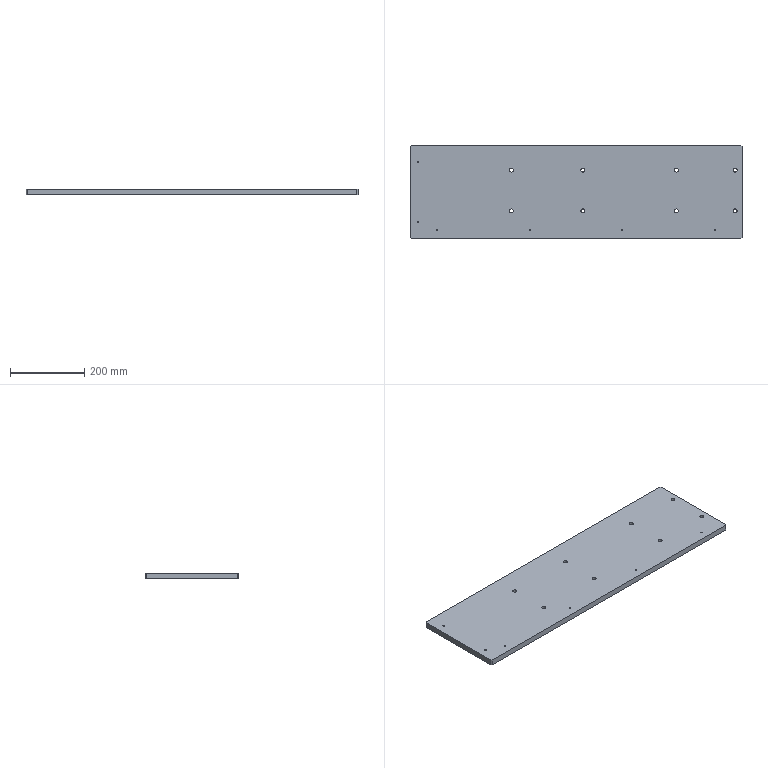Part | NX | features BREP 1 | 1 solid | 38 faces | box 895 x 252 x 16 mm | volume 3596447 mm3 | cylinder 28 | plane 10 | commonest cylinder face diameters 10.5 x16 3.3 x12
STEP:
#1=CARTESIAN_POINT('',(-168.75,59.,16.));
#2=VERTEX_POINT('',#1);
#3=CARTESIAN_POINT('',(-179.25,59.,16.));
#4=VERTEX_POINT('',#3);
#5=CARTESIAN_POINT('',(-174.,59.,16.));
#6=DIRECTION('',(0.,0.,-1.));
#7=DIRECTION('',(-1.,0.,0.));
#8=AXIS2_PLACEMENT_3D('',#5,#6,#7);
#9=CIRCLE('',#8,5.25);
#10=EDGE_CURVE('',#2,#4,#9,.T.);
#11=ORIENTED_EDGE('',*,*,#10,.F.);
#12=CARTESIAN_POINT('',(-168.75,59.,0.));
#13=VERTEX_POINT('',#12);
#14=CARTESIAN_POINT('',(-168.75,59.,0.));
#15=DIRECTION('',(0.,0.,-1.));
#16=VECTOR('',#15,1000.);
#17=LINE('',#14,#16);
#18=EDGE_CURVE('',#2,#13,#17,.T.);
#19=ORIENTED_EDGE('',*,*,#18,.T.);
#20=CARTESIAN_POINT('',(-179.25,59.,0.));
#21=VERTEX_POINT('',#20);
#22=CARTESIAN_POINT('',(-174.,59.,0.));
#23=DIRECTION('',(0.,0.,-1.));
#24=DIRECTION('',(-1.,0.,0.));
#25=AXIS2_PLACEMENT_3D('',#22,#23,#24);
#26=CIRCLE('',#25,5.25);
#27=EDGE_CURVE('',#13,#21,#26,.T.);
#28=ORIENTED_EDGE('',*,*,#27,.T.);
#29=CARTESIAN_POINT('',(-179.25,59.,0.));
#30=DIRECTION('',(0.,0.,-1.));
#31=VECTOR('',#30,1000.);
#32=LINE('',#29,#31);
#33=EDGE_CURVE('',#4,#21,#32,.T.);
#34=ORIENTED_EDGE('',*,*,#33,.F.);
#35=EDGE_LOOP('',(#11,#19,#28,#34));
#36=FACE_BOUND('',#35,.T.);
#37=CARTESIAN_POINT('',(-174.,59.,0.));
#38=DIRECTION('',(0.,0.,-1.));
#39=DIRECTION('',(-1.,0.,0.));
#40=AXIS2_PLACEMENT_3D('',#37,#38,#39);
#41=CYLINDRICAL_SURFACE('',#40,5.25);
#42=ADVANCED_FACE('',(#36),#41,.F.);
#43=CARTESIAN_POINT('',(-168.75,-51.,16.));
#44=VERTEX_POINT('',#43);
#45=CARTESIAN_POINT('',(-179.25,-51.,16.));
#46=VERTEX_POINT('',#45);
#47=CARTESIAN_POINT('',(-174.,-51.,16.));
#48=DIRECTION('',(0.,0.,-1.));
#49=DIRECTION('',(-1.,0.,0.));
#50=AXIS2_PLACEMENT_3D('',#47,#48,#49);
#51=CIRCLE('',#50,5.25);
#52=EDGE_CURVE('',#44,#46,#51,.T.);
#53=ORIENTED_EDGE('',*,*,#52,.F.);
#54=CARTESIAN_POINT('',(-168.75,-51.,0.));
#55=VERTEX_POINT('',#54);
#56=CARTESIAN_POINT('',(-168.75,-51.,0.));
#57=DIRECTION('',(0.,0.,-1.));
#58=VECTOR('',#57,1000.);
#59=LINE('',#56,#58);
#60=EDGE_CURVE('',#44,#55,#59,.T.);
#61=ORIENTED_EDGE('',*,*,#60,.T.);
#62=CARTESIAN_POINT('',(-179.25,-51.,0.));
#63=VERTEX_POINT('',#62);
#64=CARTESIAN_POINT('',(-174.,-51.,0.));
#65=DIRECTION('',(0.,0.,-1.));
#66=DIRECTION('',(-1.,0.,0.));
#67=AXIS2_PLACEMENT_3D('',#64,#65,#66);
#68=CIRCLE('',#67,5.25);
#69=EDGE_CURVE('',#55,#63,#68,.T.);
#70=ORIENTED_EDGE('',*,*,#69,.T.);
#71=CARTESIAN_POINT('',(-179.25,-51.,0.));
#72=DIRECTION('',(0.,0.,-1.));
#73=VECTOR('',#72,1000.);
#74=LINE('',#71,#73);
#75=EDGE_CURVE('',#46,#63,#74,.T.);
#76=ORIENTED_EDGE('',*,*,#75,.F.);
#77=EDGE_LOOP('',(#53,#61,#70,#76));
#78=FACE_BOUND('',#77,.T.);
#79=CARTESIAN_POINT('',(-174.,-51.,0.));
#80=DIRECTION('',(0.,0.,-1.));
#81=DIRECTION('',(-1.,0.,0.));
#82=AXIS2_PLACEMENT_3D('',#79,#80,#81);
#83=CYLINDRICAL_SURFACE('',#82,5.25);
#84=ADVANCED_FACE('',(#78),#83,.F.);
#85=CARTESIAN_POINT('',(23.75,59.,16.));
#86=VERTEX_POINT('',#85);
#87=CARTESIAN_POINT('',(13.25,59.,16.));
#88=VERTEX_POINT('',#87);
#89=CARTESIAN_POINT('',(18.5,59.,16.));
#90=DIRECTION('',(0.,0.,-1.));
#91=DIRECTION('',(-1.,0.,0.));
#92=AXIS2_PLACEMENT_3D('',#89,#90,#91);
#93=CIRCLE('',#92,5.25);
#94=EDGE_CURVE('',#86,#88,#93,.T.);
#95=ORIENTED_EDGE('',*,*,#94,.F.);
#96=CARTESIAN_POINT('',(23.75,59.,0.));
#97=VERTEX_POINT('',#96);
#98=CARTESIAN_POINT('',(23.75,59.,0.));
#99=DIRECTION('',(0.,0.,-1.));
#100=VECTOR('',#99,1000.);
#101=LINE('',#98,#100);
#102=EDGE_CURVE('',#86,#97,#101,.T.);
#103=ORIENTED_EDGE('',*,*,#102,.T.);
#104=CARTESIAN_POINT('',(13.25,59.,0.));
#105=VERTEX_POINT('',#104);
#106=CARTESIAN_POINT('',(18.5,59.,0.));
#107=DIRECTION('',(0.,0.,-1.));
#108=DIRECTION('',(-1.,0.,0.));
#109=AXIS2_PLACEMENT_3D('',#106,#107,#108);
#110=CIRCLE('',#109,5.25);
#111=EDGE_CURVE('',#97,#105,#110,.T.);
#112=ORIENTED_EDGE('',*,*,#111,.T.);
#113=CARTESIAN_POINT('',(13.25,59.,0.));
#114=DIRECTION('',(0.,0.,-1.));
#115=VECTOR('',#114,1000.);
#116=LINE('',#113,#115);
#117=EDGE_CURVE('',#88,#105,#116,.T.);
#118=ORIENTED_EDGE('',*,*,#117,.F.);
#119=EDGE_LOOP('',(#95,#103,#112,#118));
#120=FACE_BOUND('',#119,.T.);
#121=CARTESIAN_POINT('',(18.5,59.,0.));
#122=DIRECTION('',(0.,0.,-1.));
#123=DIRECTION('',(-1.,0.,0.));
#124=AXIS2_PLACEMENT_3D('',#121,#122,#123);
#125=CYLINDRICAL_SURFACE('',#124,5.25);
#126=ADVANCED_FACE('',(#120),#125,.F.);
#127=CARTESIAN_POINT('',(23.75,-51.,16.));
#128=VERTEX_POINT('',#127);
#129=CARTESIAN_POINT('',(13.25,-51.,16.));
#130=VERTEX_POINT('',#129);
#131=CARTESIAN_POINT('',(18.5,-51.,16.));
#132=DIRECTION('',(0.,0.,-1.));
#133=DIRECTION('',(-1.,0.,0.));
#134=AXIS2_PLACEMENT_3D('',#131,#132,#133);
#135=CIRCLE('',#134,5.25);
#136=EDGE_CURVE('',#128,#130,#135,.T.);
#137=ORIENTED_EDGE('',*,*,#136,.F.);
#138=CARTESIAN_POINT('',(23.75,-51.,0.));
#139=VERTEX_POINT('',#138);
#140=CARTESIAN_POINT('',(23.75,-51.,0.));
#141=DIRECTION('',(0.,0.,-1.));
#142=VECTOR('',#141,1000.);
#143=LINE('',#140,#142);
#144=EDGE_CURVE('',#128,#139,#143,.T.);
#145=ORIENTED_EDGE('',*,*,#144,.T.);
#146=CARTESIAN_POINT('',(13.25,-51.,0.));
#147=VERTEX_POINT('',#146);
#148=CARTESIAN_POINT('',(18.5,-51.,0.));
#149=DIRECTION('',(0.,0.,-1.));
#150=DIRECTION('',(-1.,0.,0.));
#151=AXIS2_PLACEMENT_3D('',#148,#149,#150);
#152=CIRCLE('',#151,5.25);
#153=EDGE_CURVE('',#139,#147,#152,.T.);
#154=ORIENTED_EDGE('',*,*,#153,.T.);
#155=CARTESIAN_POINT('',(13.25,-51.,0.));
#156=DIRECTION('',(0.,0.,-1.));
#157=VECTOR('',#156,1000.);
#158=LINE('',#155,#157);
#159=EDGE_CURVE('',#130,#147,#158,.T.);
#160=ORIENTED_EDGE('',*,*,#159,.F.);
#161=EDGE_LOOP('',(#137,#145,#154,#160));
#162=FACE_BOUND('',#161,.T.);
#163=CARTESIAN_POINT('',(18.5,-51.,0.));
#164=DIRECTION('',(0.,0.,-1.));
#165=DIRECTION('',(-1.,0.,0.));
#166=AXIS2_PLACEMENT_3D('',#163,#164,#165);
#167=CYLINDRICAL_SURFACE('',#166,5.25);
#168=ADVANCED_FACE('',(#162),#167,.F.);
#169=CARTESIAN_POINT('',(275.75,59.,16.));
#170=VERTEX_POINT('',#169);
#171=CARTESIAN_POINT('',(265.25,59.,16.));
#172=VERTEX_POINT('',#171);
#173=CARTESIAN_POINT('',(270.5,59.,16.));
#174=DIRECTION('',(0.,0.,-1.));
#175=DIRECTION('',(-1.,0.,0.));
#176=AXIS2_PLACEMENT_3D('',#173,#174,#175);
#177=CIRCLE('',#176,5.25);
#178=EDGE_CURVE('',#170,#172,#177,.T.);
#179=ORIENTED_EDGE('',*,*,#178,.F.);
#180=CARTESIAN_POINT('',(275.75,59.,0.));
#181=VERTEX_POINT('',#180);
#182=CARTESIAN_POINT('',(275.75,59.,0.));
#183=DIRECTION('',(0.,0.,-1.));
#184=VECTOR('',#183,1000.);
#185=LINE('',#182,#184);
#186=EDGE_CURVE('',#170,#181,#185,.T.);
#187=ORIENTED_EDGE('',*,*,#186,.T.);
#188=CARTESIAN_POINT('',(265.25,59.,0.));
#189=VERTEX_POINT('',#188);
#190=CARTESIAN_POINT('',(270.5,59.,0.));
#191=DIRECTION('',(0.,0.,-1.));
#192=DIRECTION('',(-1.,0.,0.));
#193=AXIS2_PLACEMENT_3D('',#190,#191,#192);
#194=CIRCLE('',#193,5.25);
#195=EDGE_CURVE('',#181,#189,#194,.T.);
#196=ORIENTED_EDGE('',*,*,#195,.T.);
#197=CARTESIAN_POINT('',(265.25,59.,0.));
#198=DIRECTION('',(0.,0.,-1.));
#199=VECTOR('',#198,1000.);
#200=LINE('',#197,#199);
#201=EDGE_CURVE('',#172,#189,#200,.T.);
#202=ORIENTED_EDGE('',*,*,#201,.F.);
#203=EDGE_LOOP('',(#179,#187,#196,#202));
#204=FACE_BOUND('',#203,.T.);
#205=CARTESIAN_POINT('',(270.5,59.,0.));
#206=DIRECTION('',(0.,0.,-1.));
#207=DIRECTION('',(-1.,0.,0.));
#208=AXIS2_PLACEMENT_3D('',#205,#206,#207);
#209=CYLINDRICAL_SURFACE('',#208,5.25);
#210=ADVANCED_FACE('',(#204),#209,.F.);
#211=CARTESIAN_POINT('',(275.75,-51.,16.));
#212=VERTEX_POINT('',#211);
#213=CARTESIAN_POINT('',(265.25,-51.,16.));
#214=VERTEX_POINT('',#213);
#215=CARTESIAN_POINT('',(270.5,-51.,16.));
#216=DIRECTION('',(0.,0.,-1.));
#217=DIRECTION('',(-1.,0.,0.));
#218=AXIS2_PLACEMENT_3D('',#215,#216,#217);
#219=CIRCLE('',#218,5.25);
#220=EDGE_CURVE('',#212,#214,#219,.T.);
#221=ORIENTED_EDGE('',*,*,#220,.F.);
#222=CARTESIAN_POINT('',(275.75,-51.,0.));
#223=VERTEX_POINT('',#222);
#224=CARTESIAN_POINT('',(275.75,-51.,0.));
#225=DIRECTION('',(0.,0.,-1.));
#226=VECTOR('',#225,1000.);
#227=LINE('',#224,#226);
#228=EDGE_CURVE('',#212,#223,#227,.T.);
#229=ORIENTED_EDGE('',*,*,#228,.T.);
#230=CARTESIAN_POINT('',(265.25,-51.,0.));
#231=VERTEX_POINT('',#230);
#232=CARTESIAN_POINT('',(270.5,-51.,0.));
#233=DIRECTION('',(0.,0.,-1.));
#234=DIRECTION('',(-1.,0.,0.));
#235=AXIS2_PLACEMENT_3D('',#232,#233,#234);
#236=CIRCLE('',#235,5.25);
#237=EDGE_CURVE('',#223,#231,#236,.T.);
#238=ORIENTED_EDGE('',*,*,#237,.T.);
#239=CARTESIAN_POINT('',(265.25,-51.,0.));
#240=DIRECTION('',(0.,0.,-1.));
#241=VECTOR('',#240,1000.);
#242=LINE('',#239,#241);
#243=EDGE_CURVE('',#214,#231,#242,.T.);
#244=ORIENTED_EDGE('',*,*,#243,.F.);
#245=EDGE_LOOP('',(#221,#229,#238,#244));
#246=FACE_BOUND('',#245,.T.);
#247=CARTESIAN_POINT('',(270.5,-51.,0.));
#248=DIRECTION('',(0.,0.,-1.));
#249=DIRECTION('',(-1.,0.,0.));
#250=AXIS2_PLACEMENT_3D('',#247,#248,#249);
#251=CYLINDRICAL_SURFACE('',#250,5.25);
#252=ADVANCED_FACE('',(#246),#251,.F.);
#253=CARTESIAN_POINT('',(434.25,-51.,16.));
#254=VERTEX_POINT('',#253);
#255=CARTESIAN_POINT('',(423.75,-51.,16.));
#256=VERTEX_POINT('',#255);
#257=CARTESIAN_POINT('',(429.,-51.,16.));
#258=DIRECTION('',(0.,0.,-1.));
#259=DIRECTION('',(-1.,0.,0.));
#260=AXIS2_PLACEMENT_3D('',#257,#258,#259);
#261=CIRCLE('',#260,5.25);
#262=EDGE_CURVE('',#254,#256,#261,.T.);
#263=ORIENTED_EDGE('',*,*,#262,.F.);
#264=CARTESIAN_POINT('',(434.25,-51.,0.));
#265=VERTEX_POINT('',#264);
#266=CARTESIAN_POINT('',(434.25,-51.,0.));
#267=DIRECTION('',(0.,0.,-1.));
#268=VECTOR('',#267,1000.);
#269=LINE('',#266,#268);
#270=EDGE_CURVE('',#254,#265,#269,.T.);
#271=ORIENTED_EDGE('',*,*,#270,.T.);
#272=CARTESIAN_POINT('',(423.75,-51.,0.));
#273=VERTEX_POINT('',#272);
#274=CARTESIAN_POINT('',(429.,-51.,0.));
#275=DIRECTION('',(0.,0.,-1.));
#276=DIRECTION('',(-1.,0.,0.));
#277=AXIS2_PLACEMENT_3D('',#274,#275,#276);
#278=CIRCLE('',#277,5.25);
#279=EDGE_CURVE('',#265,#273,#278,.T.);
#280=ORIENTED_EDGE('',*,*,#279,.T.);
#281=CARTESIAN_POINT('',(423.75,-51.,0.));
#282=DIRECTION('',(0.,0.,-1.));
#283=VECTOR('',#282,1000.);
#284=LINE('',#281,#283);
#285=EDGE_CURVE('',#256,#273,#284,.T.);
#286=ORIENTED_EDGE('',*,*,#285,.F.);
#287=EDGE_LOOP('',(#263,#271,#280,#286));
#288=FACE_BOUND('',#287,.T.);
#289=CARTESIAN_POINT('',(429.,-51.,0.));
#290=DIRECTION('',(0.,0.,-1.));
#291=DIRECTION('',(-1.,0.,0.));
#292=AXIS2_PLACEMENT_3D('',#289,#290,#291);
#293=CYLINDRICAL_SURFACE('',#292,5.25);
#294=ADVANCED_FACE('',(#288),#293,.F.);
#295=CARTESIAN_POINT('',(434.25,59.,16.));
#296=VERTEX_POINT('',#295);
#297=CARTESIAN_POINT('',(423.75,59.,16.));
#298=VERTEX_POINT('',#297);
#299=CARTESIAN_POINT('',(429.,59.,16.));
#300=DIRECTION('',(0.,0.,-1.));
#301=DIRECTION('',(-1.,0.,0.));
#302=AXIS2_PLACEMENT_3D('',#299,#300,#301);
#303=CIRCLE('',#302,5.25);
#304=EDGE_CURVE('',#296,#298,#303,.T.);
#305=ORIENTED_EDGE('',*,*,#304,.F.);
#306=CARTESIAN_POINT('',(434.25,59.,0.));
#307=VERTEX_POINT('',#306);
#308=CARTESIAN_POINT('',(434.25,59.,0.));
#309=DIRECTION('',(0.,0.,-1.));
#310=VECTOR('',#309,1000.);
#311=LINE('',#308,#310);
#312=EDGE_CURVE('',#296,#307,#311,.T.);
#313=ORIENTED_EDGE('',*,*,#312,.T.);
#314=CARTESIAN_POINT('',(423.75,59.,0.));
#315=VERTEX_POINT('',#314);
#316=CARTESIAN_POINT('',(429.,59.,0.));
#317=DIRECTION('',(0.,0.,-1.));
#318=DIRECTION('',(-1.,0.,0.));
#319=AXIS2_PLACEMENT_3D('',#316,#317,#318);
#320=CIRCLE('',#319,5.25);
#321=EDGE_CURVE('',#307,#315,#320,.T.);
#322=ORIENTED_EDGE('',*,*,#321,.T.);
#323=CARTESIAN_POINT('',(423.75,59.,0.));
#324=DIRECTION('',(0.,0.,-1.));
#325=VECTOR('',#324,1000.);
#326=LINE('',#323,#325);
#327=EDGE_CURVE('',#298,#315,#326,.T.);
#328=ORIENTED_EDGE('',*,*,#327,.F.);
#329=EDGE_LOOP('',(#305,#313,#322,#328));
#330=FACE_BOUND('',#329,.T.);
#331=CARTESIAN_POINT('',(429.,59.,0.));
#332=DIRECTION('',(0.,0.,-1.));
#333=DIRECTION('',(-1.,0.,0.));
#334=AXIS2_PLACEMENT_3D('',#331,#332,#333);
#335=CYLINDRICAL_SURFACE('',#334,5.25);
#336=ADVANCED_FACE('',(#330),#335,.F.);
#337=CARTESIAN_POINT('',(-373.35,-103.5,16.));
#338=VERTEX_POINT('',#337);
#339=CARTESIAN_POINT('',(-376.65,-103.5,16.));
#340=VERTEX_POINT('',#339);
#341=CARTESIAN_POINT('',(-375.,-103.5,16.));
#342=DIRECTION('',(0.,0.,-1.));
#343=DIRECTION('',(-1.,0.,0.));
#344=AXIS2_PLACEMENT_3D('',#341,#342,#343);
#345=CIRCLE('',#344,1.65);
#346=EDGE_CURVE('',#338,#340,#345,.T.);
#347=ORIENTED_EDGE('',*,*,#346,.F.);
#348=CARTESIAN_POINT('',(-373.35,-103.5,0.));
#349=VERTEX_POINT('',#348);
#350=CARTESIAN_POINT('',(-373.35,-103.5,0.));
#351=DIRECTION('',(0.,0.,-1.));
#352=VECTOR('',#351,1000.);
#353=LINE('',#350,#352);
#354=EDGE_CURVE('',#338,#349,#353,.T.);
#355=ORIENTED_EDGE('',*,*,#354,.T.);
#356=CARTESIAN_POINT('',(-376.65,-103.5,0.));
#357=VERTEX_POINT('',#356);
#358=CARTESIAN_POINT('',(-375.,-103.5,0.));
#359=DIRECTION('',(0.,0.,-1.));
#360=DIRECTION('',(-1.,0.,0.));
#361=AXIS2_PLACEMENT_3D('',#358,#359,#360);
#362=CIRCLE('',#361,1.65);
#363=EDGE_CURVE('',#349,#357,#362,.T.);
#364=ORIENTED_EDGE('',*,*,#363,.T.);
#365=CARTESIAN_POINT('',(-376.65,-103.5,0.));
#366=DIRECTION('',(0.,0.,-1.));
#367=VECTOR('',#366,1000.);
#368=LINE('',#365,#367);
#369=EDGE_CURVE('',#340,#357,#368,.T.);
#370=ORIENTED_EDGE('',*,*,#369,.F.);
#371=EDGE_LOOP('',(#347,#355,#364,#370));
#372=FACE_BOUND('',#371,.T.);
#373=CARTESIAN_POINT('',(-375.,-103.5,0.));
#374=DIRECTION('',(0.,0.,-1.));
#375=DIRECTION('',(-1.,0.,0.));
#376=AXIS2_PLACEMENT_3D('',#373,#374,#375);
#377=CYLINDRICAL_SURFACE('',#376,1.65);
#378=ADVANCED_FACE('',(#372),#377,.F.);
#379=CARTESIAN_POINT('',(-123.35,-103.5,16.));
#380=VERTEX_POINT('',#379);
#381=CARTESIAN_POINT('',(-126.65,-103.5,16.));
#382=VERTEX_POINT('',#381);
#383=CARTESIAN_POINT('',(-125.,-103.5,16.));
#384=DIRECTION('',(0.,0.,-1.));
#385=DIRECTION('',(-1.,0.,0.));
#386=AXIS2_PLACEMENT_3D('',#383,#384,#385);
#387=CIRCLE('',#386,1.65);
#388=EDGE_CURVE('',#380,#382,#387,.T.);
#389=ORIENTED_EDGE('',*,*,#388,.F.);
#390=CARTESIAN_POINT('',(-123.35,-103.5,0.));
#391=VERTEX_POINT('',#390);
#392=CARTESIAN_POINT('',(-123.35,-103.5,0.));
#393=DIRECTION('',(0.,0.,-1.));
#394=VECTOR('',#393,1000.);
#395=LINE('',#392,#394);
#396=EDGE_CURVE('',#380,#391,#395,.T.);
#397=ORIENTED_EDGE('',*,*,#396,.T.);
#398=CARTESIAN_POINT('',(-126.65,-103.5,0.));
#399=VERTEX_POINT('',#398);
#400=CARTESIAN_POINT('',(-125.,-103.5,0.));
#401=DIRECTION('',(0.,0.,-1.));
#402=DIRECTION('',(-1.,0.,0.));
#403=AXIS2_PLACEMENT_3D('',#400,#401,#402);
#404=CIRCLE('',#403,1.65);
#405=EDGE_CURVE('',#391,#399,#404,.T.);
#406=ORIENTED_EDGE('',*,*,#405,.T.);
#407=CARTESIAN_POINT('',(-126.65,-103.5,0.));
#408=DIRECTION('',(0.,0.,-1.));
#409=VECTOR('',#408,1000.);
#410=LINE('',#407,#409);
#411=EDGE_CURVE('',#382,#399,#410,.T.);
#412=ORIENTED_EDGE('',*,*,#411,.F.);
#413=EDGE_LOOP('',(#389,#397,#406,#412));
#414=FACE_BOUND('',#413,.T.);
#415=CARTESIAN_POINT('',(-125.,-103.5,0.));
#416=DIRECTION('',(0.,0.,-1.));
#417=DIRECTION('',(-1.,0.,0.));
#418=AXIS2_PLACEMENT_3D('',#415,#416,#417);
#419=CYLINDRICAL_SURFACE('',#418,1.65);
#420=ADVANCED_FACE('',(#414),#419,.F.);
#421=CARTESIAN_POINT('',(126.65,-103.5,16.));
#422=VERTEX_POINT('',#421);
#423=CARTESIAN_POINT('',(123.35,-103.5,16.));
#424=VERTEX_POINT('',#423);
#425=CARTESIAN_POINT('',(125.,-103.5,16.));
#426=DIRECTION('',(0.,0.,-1.));
#427=DIRECTION('',(-1.,0.,0.));
#428=AXIS2_PLACEMENT_3D('',#425,#426,#427);
#429=CIRCLE('',#428,1.65);
#430=EDGE_CURVE('',#422,#424,#429,.T.);
#431=ORIENTED_EDGE('',*,*,#430,.F.);
#432=CARTESIAN_POINT('',(126.65,-103.5,0.));
#433=VERTEX_POINT('',#432);
#434=CARTESIAN_POINT('',(126.65,-103.5,0.));
#435=DIRECTION('',(0.,0.,-1.));
#436=VECTOR('',#435,1000.);
#437=LINE('',#434,#436);
#438=EDGE_CURVE('',#422,#433,#437,.T.);
#439=ORIENTED_EDGE('',*,*,#438,.T.);
#440=CARTESIAN_POINT('',(123.35,-103.5,0.));
#441=VERTEX_POINT('',#440);
#442=CARTESIAN_POINT('',(125.,-103.5,0.));
#443=DIRECTION('',(0.,0.,-1.));
#444=DIRECTION('',(-1.,0.,0.));
#445=AXIS2_PLACEMENT_3D('',#442,#443,#444);
#446=CIRCLE('',#445,1.65);
#447=EDGE_CURVE('',#433,#441,#446,.T.);
#448=ORIENTED_EDGE('',*,*,#447,.T.);
#449=CARTESIAN_POINT('',(123.35,-103.5,0.));
#450=DIRECTION('',(0.,0.,-1.));
#451=VECTOR('',#450,1000.);
#452=LINE('',#449,#451);
#453=EDGE_CURVE('',#424,#441,#452,.T.);
#454=ORIENTED_EDGE('',*,*,#453,.F.);
#455=EDGE_LOOP('',(#431,#439,#448,#454));
#456=FACE_BOUND('',#455,.T.);
#457=CARTESIAN_POINT('',(125.,-103.5,0.));
#458=DIRECTION('',(0.,0.,-1.));
#459=DIRECTION('',(-1.,0.,0.));
#460=AXIS2_PLACEMENT_3D('',#457,#458,#459);
#461=CYLINDRICAL_SURFACE('',#460,1.65);
#462=ADVANCED_FACE('',(#456),#461,.F.);
#463=CARTESIAN_POINT('',(376.65,-103.5,16.));
#464=VERTEX_POINT('',#463);
#465=CARTESIAN_POINT('',(373.35,-103.5,16.));
#466=VERTEX_POINT('',#465);
#467=CARTESIAN_POINT('',(375.,-103.5,16.));
#468=DIRECTION('',(0.,0.,-1.));
#469=DIRECTION('',(-1.,0.,0.));
#470=AXIS2_PLACEMENT_3D('',#467,#468,#469);
#471=CIRCLE('',#470,1.65);
#472=EDGE_CURVE('',#464,#466,#471,.T.);
#473=ORIENTED_EDGE('',*,*,#472,.F.);
#474=CARTESIAN_POINT('',(376.65,-103.5,0.));
#475=VERTEX_POINT('',#474);
#476=CARTESIAN_POINT('',(376.65,-103.5,0.));
#477=DIRECTION('',(0.,0.,-1.));
#478=VECTOR('',#477,1000.);
#479=LINE('',#476,#478);
#480=EDGE_CURVE('',#464,#475,#479,.T.);
#481=ORIENTED_EDGE('',*,*,#480,.T.);
#482=CARTESIAN_POINT('',(373.35,-103.5,0.));
#483=VERTEX_POINT('',#482);
#484=CARTESIAN_POINT('',(375.,-103.5,0.));
#485=DIRECTION('',(0.,0.,-1.));
#486=DIRECTION('',(-1.,0.,0.));
#487=AXIS2_PLACEMENT_3D('',#484,#485,#486);
#488=CIRCLE('',#487,1.65);
#489=EDGE_CURVE('',#475,#483,#488,.T.);
#490=ORIENTED_EDGE('',*,*,#489,.T.);
#491=CARTESIAN_POINT('',(373.35,-103.5,0.));
#492=DIRECTION('',(0.,0.,-1.));
#493=VECTOR('',#492,1000.);
#494=LINE('',#491,#493);
#495=EDGE_CURVE('',#466,#483,#494,.T.);
#496=ORIENTED_EDGE('',*,*,#495,.F.);
#497=EDGE_LOOP('',(#473,#481,#490,#496));
#498=FACE_BOUND('',#497,.T.);
#499=CARTESIAN_POINT('',(375.,-103.5,0.));
#500=DIRECTION('',(0.,0.,-1.));
#501=DIRECTION('',(-1.,0.,0.));
#502=AXIS2_PLACEMENT_3D('',#499,#500,#501);
#503=CYLINDRICAL_SURFACE('',#502,1.65);
#504=ADVANCED_FACE('',(#498),#503,.F.);
#505=CARTESIAN_POINT('',(-423.35,-80.,16.));
#506=VERTEX_POINT('',#505);
#507=CARTESIAN_POINT('',(-426.65,-80.,16.));
#508=VERTEX_POINT('',#507);
#509=CARTESIAN_POINT('',(-425.,-80.,16.));
#510=DIRECTION('',(0.,0.,-1.));
#511=DIRECTION('',(-1.,0.,0.));
#512=AXIS2_PLACEMENT_3D('',#509,#510,#511);
#513=CIRCLE('',#512,1.65);
#514=EDGE_CURVE('',#506,#508,#513,.T.);
#515=ORIENTED_EDGE('',*,*,#514,.F.);
#516=CARTESIAN_POINT('',(-423.35,-80.,0.));
#517=VERTEX_POINT('',#516);
#518=CARTESIAN_POINT('',(-423.35,-80.,0.));
#519=DIRECTION('',(0.,0.,-1.));
#520=VECTOR('',#519,1000.);
#521=LINE('',#518,#520);
#522=EDGE_CURVE('',#506,#517,#521,.T.);
#523=ORIENTED_EDGE('',*,*,#522,.T.);
#524=CARTESIAN_POINT('',(-426.65,-80.,0.));
#525=VERTEX_POINT('',#524);
#526=CARTESIAN_POINT('',(-425.,-80.,0.));
#527=DIRECTION('',(0.,0.,-1.));
#528=DIRECTION('',(-1.,0.,0.));
#529=AXIS2_PLACEMENT_3D('',#526,#527,#528);
#530=CIRCLE('',#529,1.65);
#531=EDGE_CURVE('',#517,#525,#530,.T.);
#532=ORIENTED_EDGE('',*,*,#531,.T.);
#533=CARTESIAN_POINT('',(-426.65,-80.,0.));
#534=DIRECTION('',(0.,0.,-1.));
#535=VECTOR('',#534,1000.);
#536=LINE('',#533,#535);
#537=EDGE_CURVE('',#508,#525,#536,.T.);
#538=ORIENTED_EDGE('',*,*,#537,.F.);
#539=EDGE_LOOP('',(#515,#523,#532,#538));
#540=FACE_BOUND('',#539,.T.);
#541=CARTESIAN_POINT('',(-425.,-80.,0.));
#542=DIRECTION('',(0.,0.,-1.));
#543=DIRECTION('',(-1.,0.,0.));
#544=AXIS2_PLACEMENT_3D('',#541,#542,#543);
#545=CYLINDRICAL_SURFACE('',#544,1.65);
#546=ADVANCED_FACE('',(#540),#545,.F.);
#547=CARTESIAN_POINT('',(-423.35,80.,16.));
#548=VERTEX_POINT('',#547);
#549=CARTESIAN_POINT('',(-426.65,80.,16.));
#550=VERTEX_POINT('',#549);
#551=CARTESIAN_POINT('',(-425.,80.,16.));
#552=DIRECTION('',(0.,0.,-1.));
#553=DIRECTION('',(-1.,0.,0.));
#554=AXIS2_PLACEMENT_3D('',#551,#552,#553);
#555=CIRCLE('',#554,1.65);
#556=EDGE_CURVE('',#548,#550,#555,.T.);
#557=ORIENTED_EDGE('',*,*,#556,.F.);
#558=CARTESIAN_POINT('',(-423.35,80.,0.));
#559=VERTEX_POINT('',#558);
#560=CARTESIAN_POINT('',(-423.35,80.,0.));
#561=DIRECTION('',(0.,0.,-1.));
#562=VECTOR('',#561,1000.);
#563=LINE('',#560,#562);
#564=EDGE_CURVE('',#548,#559,#563,.T.);
#565=ORIENTED_EDGE('',*,*,#564,.T.);
#566=CARTESIAN_POINT('',(-426.65,80.,0.));
#567=VERTEX_POINT('',#566);
#568=CARTESIAN_POINT('',(-425.,80.,0.));
#569=DIRECTION('',(0.,0.,-1.));
#570=DIRECTION('',(-1.,0.,0.));
#571=AXIS2_PLACEMENT_3D('',#568,#569,#570);
#572=CIRCLE('',#571,1.65);
#573=EDGE_CURVE('',#559,#567,#572,.T.);
#574=ORIENTED_EDGE('',*,*,#573,.T.);
#575=CARTESIAN_POINT('',(-426.65,80.,0.));
#576=DIRECTION('',(0.,0.,-1.));
#577=VECTOR('',#576,1000.);
#578=LINE('',#575,#577);
#579=EDGE_CURVE('',#550,#567,#578,.T.);
#580=ORIENTED_EDGE('',*,*,#579,.F.);
#581=EDGE_LOOP('',(#557,#565,#574,#580));
#582=FACE_BOUND('',#581,.T.);
#583=CARTESIAN_POINT('',(-425.,80.,0.));
#584=DIRECTION('',(0.,0.,-1.));
#585=DIRECTION('',(-1.,0.,0.));
#586=AXIS2_PLACEMENT_3D('',#583,#584,#585);
#587=CYLINDRICAL_SURFACE('',#586,1.65);
#588=ADVANCED_FACE('',(#582),#587,.F.);
#589=CARTESIAN_POINT('',(447.5,-123.,16.));
#590=VERTEX_POINT('',#589);
#591=CARTESIAN_POINT('',(447.5,123.,16.));
#592=VERTEX_POINT('',#591);
#593=CARTESIAN_POINT('',(447.5,126.,16.));
#594=DIRECTION('',(0.,1.,0.));
#595=VECTOR('',#594,1000.);
#596=LINE('',#593,#595);
#597=EDGE_CURVE('',#590,#592,#596,.T.);
#598=ORIENTED_EDGE('',*,*,#597,.F.);
#599=CARTESIAN_POINT('',(447.5,-123.,0.));
#600=VERTEX_POINT('',#599);
#601=CARTESIAN_POINT('',(447.5,-123.,16.));
#602=DIRECTION('',(0.,0.,-1.));
#603=VECTOR('',#602,1000.);
#604=LINE('',#601,#603);
#605=EDGE_CURVE('',#590,#600,#604,.T.);
#606=ORIENTED_EDGE('',*,*,#605,.T.);
#607=CARTESIAN_POINT('',(447.5,123.,0.));
#608=VERTEX_POINT('',#607);
#609=CARTESIAN_POINT('',(447.5,126.,0.));
#610=DIRECTION('',(0.,1.,0.));
#611=VECTOR('',#610,1000.);
#612=LINE('',#609,#611);
#613=EDGE_CURVE('',#600,#608,#612,.T.);
#614=ORIENTED_EDGE('',*,*,#613,.T.);
#615=CARTESIAN_POINT('',(447.5,123.,16.));
#616=DIRECTION('',(0.,0.,1.));
#617=VECTOR('',#616,1000.);
#618=LINE('',#615,#617);
#619=EDGE_CURVE('',#608,#592,#618,.T.);
#620=ORIENTED_EDGE('',*,*,#619,.T.);
#621=EDGE_LOOP('',(#598,#606,#614,#620));
#622=FACE_BOUND('',#621,.T.);
#623=CARTESIAN_POINT('',(447.5,126.,16.));
#624=DIRECTION('',(-1.,0.,0.));
#625=DIRECTION('',(0.,0.,1.));
#626=AXIS2_PLACEMENT_3D('',#623,#624,#625);
#627=PLANE('',#626);
#628=ADVANCED_FACE('',(#622),#627,.F.);
#629=CARTESIAN_POINT('',(444.5,126.,0.));
#630=VERTEX_POINT('',#629);
#631=CARTESIAN_POINT('',(-444.5,126.,0.));
#632=VERTEX_POINT('',#631);
#633=CARTESIAN_POINT('',(-447.5,126.,0.));
#634=DIRECTION('',(-1.,0.,0.));
#635=VECTOR('',#634,1000.);
#636=LINE('',#633,#635);
#637=EDGE_CURVE('',#630,#632,#636,.T.);
#638=ORIENTED_EDGE('',*,*,#637,.T.);
#639=CARTESIAN_POINT('',(-444.5,126.,16.));
#640=VERTEX_POINT('',#639);
#641=CARTESIAN_POINT('',(-444.5,126.,16.));
#642=DIRECTION('',(0.,0.,1.));
#643=VECTOR('',#642,1000.);
#644=LINE('',#641,#643);
#645=EDGE_CURVE('',#632,#640,#644,.T.);
#646=ORIENTED_EDGE('',*,*,#645,.T.);
#647=CARTESIAN_POINT('',(444.5,126.,16.));
#648=VERTEX_POINT('',#647);
#649=CARTESIAN_POINT('',(-447.5,126.,16.));
#650=DIRECTION('',(-1.,0.,0.));
#651=VECTOR('',#650,1000.);
#652=LINE('',#649,#651);
#653=EDGE_CURVE('',#648,#640,#652,.T.);
#654=ORIENTED_EDGE('',*,*,#653,.F.);
#655=CARTESIAN_POINT('',(444.5,126.,16.));
#656=DIRECTION('',(0.,0.,-1.));
#657=VECTOR('',#656,1000.);
#658=LINE('',#655,#657);
#659=EDGE_CURVE('',#648,#630,#658,.T.);
#660=ORIENTED_EDGE('',*,*,#659,.T.);
#661=EDGE_LOOP('',(#638,#646,#654,#660));
#662=FACE_BOUND('',#661,.T.);
#663=CARTESIAN_POINT('',(-447.5,126.,16.));
#664=DIRECTION('',(0.,-1.,0.));
#665=DIRECTION('',(0.,0.,-1.));
#666=AXIS2_PLACEMENT_3D('',#663,#664,#665);
#667=PLANE('',#666);
#668=ADVANCED_FACE('',(#662),#667,.F.);
#669=CARTESIAN_POINT('',(-447.5,123.,0.));
#670=VERTEX_POINT('',#669);
#671=CARTESIAN_POINT('',(-447.5,-123.,0.));
#672=VERTEX_POINT('',#671);
#673=CARTESIAN_POINT('',(-447.5,126.,0.));
#674=DIRECTION('',(0.,-1.,0.));
#675=VECTOR('',#674,1000.);
#676=LINE('',#673,#675);
#677=EDGE_CURVE('',#670,#672,#676,.T.);
#678=ORIENTED_EDGE('',*,*,#677,.T.);
#679=CARTESIAN_POINT('',(-447.5,-123.,16.));
#680=VERTEX_POINT('',#679);
#681=CARTESIAN_POINT('',(-447.5,-123.,16.));
#682=DIRECTION('',(0.,0.,1.));
#683=VECTOR('',#682,1000.);
#684=LINE('',#681,#683);
#685=EDGE_CURVE('',#672,#680,#684,.T.);
#686=ORIENTED_EDGE('',*,*,#685,.T.);
#687=CARTESIAN_POINT('',(-447.5,123.,16.));
#688=VERTEX_POINT('',#687);
#689=CARTESIAN_POINT('',(-447.5,126.,16.));
#690=DIRECTION('',(0.,-1.,0.));
#691=VECTOR('',#690,1000.);
#692=LINE('',#689,#691);
#693=EDGE_CURVE('',#688,#680,#692,.T.);
#694=ORIENTED_EDGE('',*,*,#693,.F.);
#695=CARTESIAN_POINT('',(-447.5,123.,16.));
#696=DIRECTION('',(0.,0.,-1.));
#697=VECTOR('',#696,1000.);
#698=LINE('',#695,#697);
#699=EDGE_CURVE('',#688,#670,#698,.T.);
#700=ORIENTED_EDGE('',*,*,#699,.T.);
#701=EDGE_LOOP('',(#678,#686,#694,#700));
#702=FACE_BOUND('',#701,.T.);
#703=CARTESIAN_POINT('',(-447.5,126.,16.));
#704=DIRECTION('',(1.,0.,0.));
#705=DIRECTION('',(0.,1.,0.));
#706=AXIS2_PLACEMENT_3D('',#703,#704,#705);
#707=PLANE('',#706);
#708=ADVANCED_FACE('',(#702),#707,.F.);
#709=CARTESIAN_POINT('',(-444.5,-126.,0.));
#710=VERTEX_POINT('',#709);
#711=CARTESIAN_POINT('',(444.5,-126.,0.));
#712=VERTEX_POINT('',#711);
#713=CARTESIAN_POINT('',(-447.5,-126.,0.));
#714=DIRECTION('',(1.,0.,0.));
#715=VECTOR('',#714,1000.);
#716=LINE('',#713,#715);
#717=EDGE_CURVE('',#710,#712,#716,.T.);
#718=ORIENTED_EDGE('',*,*,#717,.T.);
#719=CARTESIAN_POINT('',(444.5,-126.,16.));
#720=VERTEX_POINT('',#719);
#721=CARTESIAN_POINT('',(444.5,-126.,16.));
#722=DIRECTION('',(0.,0.,1.));
#723=VECTOR('',#722,1000.);
#724=LINE('',#721,#723);
#725=EDGE_CURVE('',#712,#720,#724,.T.);
#726=ORIENTED_EDGE('',*,*,#725,.T.);
#727=CARTESIAN_POINT('',(-444.5,-126.,16.));
#728=VERTEX_POINT('',#727);
#729=CARTESIAN_POINT('',(-447.5,-126.,16.));
#730=DIRECTION('',(1.,0.,0.));
#731=VECTOR('',#730,1000.);
#732=LINE('',#729,#731);
#733=EDGE_CURVE('',#728,#720,#732,.T.);
#734=ORIENTED_EDGE('',*,*,#733,.F.);
#735=CARTESIAN_POINT('',(-444.5,-126.,16.));
#736=DIRECTION('',(0.,0.,-1.));
#737=VECTOR('',#736,1000.);
#738=LINE('',#735,#737);
#739=EDGE_CURVE('',#728,#710,#738,.T.);
#740=ORIENTED_EDGE('',*,*,#739,.T.);
#741=EDGE_LOOP('',(#718,#726,#734,#740));
#742=FACE_BOUND('',#741,.T.);
#743=CARTESIAN_POINT('',(-447.5,-126.,16.));
#744=DIRECTION('',(0.,1.,0.));
#745=DIRECTION('',(1.,0.,0.));
#746=AXIS2_PLACEMENT_3D('',#743,#744,#745);
#747=PLANE('',#746);
#748=ADVANCED_FACE('',(#742),#747,.F.);
#749=ORIENTED_EDGE('',*,*,#733,.T.);
#750=CARTESIAN_POINT('',(446.,-124.5,16.));
#751=DIRECTION('',(0.7071,0.7071,0.));
#752=VECTOR('',#751,1000.);
#753=LINE('',#750,#752);
#754=EDGE_CURVE('',#720,#590,#753,.T.);
#755=ORIENTED_EDGE('',*,*,#754,.T.);
#756=ORIENTED_EDGE('',*,*,#597,.T.);
#757=CARTESIAN_POINT('',(572.,-1.5,16.));
#758=DIRECTION('',(-0.7071,0.7071,0.));
#759=VECTOR('',#758,1000.);
#760=LINE('',#757,#759);
#761=EDGE_CURVE('',#592,#648,#760,.T.);
#762=ORIENTED_EDGE('',*,*,#761,.T.);
#763=ORIENTED_EDGE('',*,*,#653,.T.);
#764=CARTESIAN_POINT('',(-124.5,446.,16.));
#765=DIRECTION('',(-0.7071,-0.7071,0.));
#766=VECTOR('',#765,1000.);
#767=LINE('',#764,#766);
#768=EDGE_CURVE('',#640,#688,#767,.T.);
#769=ORIENTED_EDGE('',*,*,#768,.T.);
#770=ORIENTED_EDGE('',*,*,#693,.T.);
#771=CARTESIAN_POINT('',(1.5,-572.,16.));
#772=DIRECTION('',(0.7071,-0.7071,0.));
#773=VECTOR('',#772,1000.);
#774=LINE('',#771,#773);
#775=EDGE_CURVE('',#680,#728,#774,.T.);
#776=ORIENTED_EDGE('',*,*,#775,.T.);
#777=EDGE_LOOP('',(#749,#755,#756,#762,#763,#769,#770,#776));
#778=FACE_BOUND('',#777,.T.);
#779=CARTESIAN_POINT('',(-174.,59.,16.));
#780=DIRECTION('',(0.,0.,-1.));
#781=DIRECTION('',(-1.,0.,0.));
#782=AXIS2_PLACEMENT_3D('',#779,#780,#781);
#783=CIRCLE('',#782,5.25);
#784=EDGE_CURVE('',#4,#2,#783,.T.);
#785=ORIENTED_EDGE('',*,*,#784,.T.);
#786=ORIENTED_EDGE('',*,*,#10,.T.);
#787=EDGE_LOOP('',(#785,#786));
#788=FACE_BOUND('',#787,.T.);
#789=CARTESIAN_POINT('',(-174.,-51.,16.));
#790=DIRECTION('',(0.,0.,-1.));
#791=DIRECTION('',(-1.,0.,0.));
#792=AXIS2_PLACEMENT_3D('',#789,#790,#791);
#793=CIRCLE('',#792,5.25);
#794=EDGE_CURVE('',#46,#44,#793,.T.);
#795=ORIENTED_EDGE('',*,*,#794,.T.);
#796=ORIENTED_EDGE('',*,*,#52,.T.);
#797=EDGE_LOOP('',(#795,#796));
#798=FACE_BOUND('',#797,.T.);
#799=CARTESIAN_POINT('',(18.5,59.,16.));
#800=DIRECTION('',(0.,0.,-1.));
#801=DIRECTION('',(-1.,0.,0.));
#802=AXIS2_PLACEMENT_3D('',#799,#800,#801);
#803=CIRCLE('',#802,5.25);
#804=EDGE_CURVE('',#88,#86,#803,.T.);
#805=ORIENTED_EDGE('',*,*,#804,.T.);
#806=ORIENTED_EDGE('',*,*,#94,.T.);
#807=EDGE_LOOP('',(#805,#806));
#808=FACE_BOUND('',#807,.T.);
#809=CARTESIAN_POINT('',(18.5,-51.,16.));
#810=DIRECTION('',(0.,0.,-1.));
#811=DIRECTION('',(-1.,0.,0.));
#812=AXIS2_PLACEMENT_3D('',#809,#810,#811);
#813=CIRCLE('',#812,5.25);
#814=EDGE_CURVE('',#130,#128,#813,.T.);
#815=ORIENTED_EDGE('',*,*,#814,.T.);
#816=ORIENTED_EDGE('',*,*,#136,.T.);
#817=EDGE_LOOP('',(#815,#816));
#818=FACE_BOUND('',#817,.T.);
#819=CARTESIAN_POINT('',(270.5,59.,16.));
#820=DIRECTION('',(0.,0.,-1.));
#821=DIRECTION('',(-1.,0.,0.));
#822=AXIS2_PLACEMENT_3D('',#819,#820,#821);
#823=CIRCLE('',#822,5.25);
#824=EDGE_CURVE('',#172,#170,#823,.T.);
#825=ORIENTED_EDGE('',*,*,#824,.T.);
#826=ORIENTED_EDGE('',*,*,#178,.T.);
#827=EDGE_LOOP('',(#825,#826));
#828=FACE_BOUND('',#827,.T.);
#829=CARTESIAN_POINT('',(270.5,-51.,16.));
#830=DIRECTION('',(0.,0.,-1.));
#831=DIRECTION('',(-1.,0.,0.));
#832=AXIS2_PLACEMENT_3D('',#829,#830,#831);
#833=CIRCLE('',#832,5.25);
#834=EDGE_CURVE('',#214,#212,#833,.T.);
#835=ORIENTED_EDGE('',*,*,#834,.T.);
#836=ORIENTED_EDGE('',*,*,#220,.T.);
#837=EDGE_LOOP('',(#835,#836));
#838=FACE_BOUND('',#837,.T.);
#839=CARTESIAN_POINT('',(429.,-51.,16.));
#840=DIRECTION('',(0.,0.,-1.));
#841=DIRECTION('',(-1.,0.,0.));
#842=AXIS2_PLACEMENT_3D('',#839,#840,#841);
#843=CIRCLE('',#842,5.25);
#844=EDGE_CURVE('',#256,#254,#843,.T.);
#845=ORIENTED_EDGE('',*,*,#844,.T.);
#846=ORIENTED_EDGE('',*,*,#262,.T.);
#847=EDGE_LOOP('',(#845,#846));
#848=FACE_BOUND('',#847,.T.);
#849=CARTESIAN_POINT('',(429.,59.,16.));
#850=DIRECTION('',(0.,0.,-1.));
#851=DIRECTION('',(-1.,0.,0.));
#852=AXIS2_PLACEMENT_3D('',#849,#850,#851);
#853=CIRCLE('',#852,5.25);
#854=EDGE_CURVE('',#298,#296,#853,.T.);
#855=ORIENTED_EDGE('',*,*,#854,.T.);
#856=ORIENTED_EDGE('',*,*,#304,.T.);
#857=EDGE_LOOP('',(#855,#856));
#858=FACE_BOUND('',#857,.T.);
#859=CARTESIAN_POINT('',(-375.,-103.5,16.));
#860=DIRECTION('',(0.,0.,-1.));
#861=DIRECTION('',(-1.,0.,0.));
#862=AXIS2_PLACEMENT_3D('',#859,#860,#861);
#863=CIRCLE('',#862,1.65);
#864=EDGE_CURVE('',#340,#338,#863,.T.);
#865=ORIENTED_EDGE('',*,*,#864,.T.);
#866=ORIENTED_EDGE('',*,*,#346,.T.);
#867=EDGE_LOOP('',(#865,#866));
#868=FACE_BOUND('',#867,.T.);
#869=CARTESIAN_POINT('',(-125.,-103.5,16.));
#870=DIRECTION('',(0.,0.,-1.));
#871=DIRECTION('',(-1.,0.,0.));
#872=AXIS2_PLACEMENT_3D('',#869,#870,#871);
#873=CIRCLE('',#872,1.65);
#874=EDGE_CURVE('',#382,#380,#873,.T.);
#875=ORIENTED_EDGE('',*,*,#874,.T.);
#876=ORIENTED_EDGE('',*,*,#388,.T.);
#877=EDGE_LOOP('',(#875,#876));
#878=FACE_BOUND('',#877,.T.);
#879=CARTESIAN_POINT('',(125.,-103.5,16.));
#880=DIRECTION('',(0.,0.,-1.));
#881=DIRECTION('',(-1.,0.,0.));
#882=AXIS2_PLACEMENT_3D('',#879,#880,#881);
#883=CIRCLE('',#882,1.65);
#884=EDGE_CURVE('',#424,#422,#883,.T.);
#885=ORIENTED_EDGE('',*,*,#884,.T.);
#886=ORIENTED_EDGE('',*,*,#430,.T.);
#887=EDGE_LOOP('',(#885,#886));
#888=FACE_BOUND('',#887,.T.);
#889=CARTESIAN_POINT('',(375.,-103.5,16.));
#890=DIRECTION('',(0.,0.,-1.));
#891=DIRECTION('',(-1.,0.,0.));
#892=AXIS2_PLACEMENT_3D('',#889,#890,#891);
#893=CIRCLE('',#892,1.65);
#894=EDGE_CURVE('',#466,#464,#893,.T.);
#895=ORIENTED_EDGE('',*,*,#894,.T.);
#896=ORIENTED_EDGE('',*,*,#472,.T.);
#897=EDGE_LOOP('',(#895,#896));
#898=FACE_BOUND('',#897,.T.);
#899=CARTESIAN_POINT('',(-425.,-80.,16.));
#900=DIRECTION('',(0.,0.,-1.));
#901=DIRECTION('',(-1.,0.,0.));
#902=AXIS2_PLACEMENT_3D('',#899,#900,#901);
#903=CIRCLE('',#902,1.65);
#904=EDGE_CURVE('',#508,#506,#903,.T.);
#905=ORIENTED_EDGE('',*,*,#904,.T.);
#906=ORIENTED_EDGE('',*,*,#514,.T.);
#907=EDGE_LOOP('',(#905,#906));
#908=FACE_BOUND('',#907,.T.);
#909=CARTESIAN_POINT('',(-425.,80.,16.));
#910=DIRECTION('',(0.,0.,-1.));
#911=DIRECTION('',(-1.,0.,0.));
#912=AXIS2_PLACEMENT_3D('',#909,#910,#911);
#913=CIRCLE('',#912,1.65);
#914=EDGE_CURVE('',#550,#548,#913,.T.);
#915=ORIENTED_EDGE('',*,*,#914,.T.);
#916=ORIENTED_EDGE('',*,*,#556,.T.);
#917=EDGE_LOOP('',(#915,#916));
#918=FACE_BOUND('',#917,.T.);
#919=CARTESIAN_POINT('',(447.5,-126.,16.));
#920=DIRECTION('',(0.,0.,1.));
#921=DIRECTION('',(1.,0.,0.));
#922=AXIS2_PLACEMENT_3D('',#919,#920,#921);
#923=PLANE('',#922);
#924=ADVANCED_FACE('',(#778,#788,#798,#808,#818,#828,#838,#848,#858,#868,#878,#888,#898,#908,#918),#923,.T.);
#925=ORIENTED_EDGE('',*,*,#613,.F.);
#926=CARTESIAN_POINT('',(447.5,-123.,0.));
#927=DIRECTION('',(-0.7071,-0.7071,0.));
#928=VECTOR('',#927,1000.);
#929=LINE('',#926,#928);
#930=EDGE_CURVE('',#600,#712,#929,.T.);
#931=ORIENTED_EDGE('',*,*,#930,.T.);
#932=ORIENTED_EDGE('',*,*,#717,.F.);
#933=CARTESIAN_POINT('',(-444.5,-126.,0.));
#934=DIRECTION('',(-0.7071,0.7071,0.));
#935=VECTOR('',#934,1000.);
#936=LINE('',#933,#935);
#937=EDGE_CURVE('',#710,#672,#936,.T.);
#938=ORIENTED_EDGE('',*,*,#937,.T.);
#939=ORIENTED_EDGE('',*,*,#677,.F.);
#940=CARTESIAN_POINT('',(-447.5,123.,0.));
#941=DIRECTION('',(0.7071,0.7071,0.));
#942=VECTOR('',#941,1000.);
#943=LINE('',#940,#942);
#944=EDGE_CURVE('',#670,#632,#943,.T.);
#945=ORIENTED_EDGE('',*,*,#944,.T.);
#946=ORIENTED_EDGE('',*,*,#637,.F.);
#947=CARTESIAN_POINT('',(444.5,126.,0.));
#948=DIRECTION('',(0.7071,-0.7071,0.));
#949=VECTOR('',#948,1000.);
#950=LINE('',#947,#949);
#951=EDGE_CURVE('',#630,#608,#950,.T.);
#952=ORIENTED_EDGE('',*,*,#951,.T.);
#953=EDGE_LOOP('',(#925,#931,#932,#938,#939,#945,#946,#952));
#954=FACE_BOUND('',#953,.T.);
#955=CARTESIAN_POINT('',(-174.,59.,0.));
#956=DIRECTION('',(0.,0.,-1.));
#957=DIRECTION('',(-1.,0.,0.));
#958=AXIS2_PLACEMENT_3D('',#955,#956,#957);
#959=CIRCLE('',#958,5.25);
#960=EDGE_CURVE('',#21,#13,#959,.T.);
#961=ORIENTED_EDGE('',*,*,#960,.F.);
#962=ORIENTED_EDGE('',*,*,#27,.F.);
#963=EDGE_LOOP('',(#961,#962));
#964=FACE_BOUND('',#963,.T.);
#965=CARTESIAN_POINT('',(-174.,-51.,0.));
#966=DIRECTION('',(0.,0.,-1.));
#967=DIRECTION('',(-1.,0.,0.));
#968=AXIS2_PLACEMENT_3D('',#965,#966,#967);
#969=CIRCLE('',#968,5.25);
#970=EDGE_CURVE('',#63,#55,#969,.T.);
#971=ORIENTED_EDGE('',*,*,#970,.F.);
#972=ORIENTED_EDGE('',*,*,#69,.F.);
#973=EDGE_LOOP('',(#971,#972));
#974=FACE_BOUND('',#973,.T.);
#975=CARTESIAN_POINT('',(18.5,59.,0.));
#976=DIRECTION('',(0.,0.,-1.));
#977=DIRECTION('',(-1.,0.,0.));
#978=AXIS2_PLACEMENT_3D('',#975,#976,#977);
#979=CIRCLE('',#978,5.25);
#980=EDGE_CURVE('',#105,#97,#979,.T.);
#981=ORIENTED_EDGE('',*,*,#980,.F.);
#982=ORIENTED_EDGE('',*,*,#111,.F.);
#983=EDGE_LOOP('',(#981,#982));
#984=FACE_BOUND('',#983,.T.);
#985=CARTESIAN_POINT('',(18.5,-51.,0.));
#986=DIRECTION('',(0.,0.,-1.));
#987=DIRECTION('',(-1.,0.,0.));
#988=AXIS2_PLACEMENT_3D('',#985,#986,#987);
#989=CIRCLE('',#988,5.25);
#990=EDGE_CURVE('',#147,#139,#989,.T.);
#991=ORIENTED_EDGE('',*,*,#990,.F.);
#992=ORIENTED_EDGE('',*,*,#153,.F.);
#993=EDGE_LOOP('',(#991,#992));
#994=FACE_BOUND('',#993,.T.);
#995=CARTESIAN_POINT('',(270.5,59.,0.));
#996=DIRECTION('',(0.,0.,-1.));
#997=DIRECTION('',(-1.,0.,0.));
#998=AXIS2_PLACEMENT_3D('',#995,#996,#997);
#999=CIRCLE('',#998,5.25);
#1000=EDGE_CURVE('',#189,#181,#999,.T.);
#1001=ORIENTED_EDGE('',*,*,#1000,.F.);
#1002=ORIENTED_EDGE('',*,*,#195,.F.);
#1003=EDGE_LOOP('',(#1001,#1002));
#1004=FACE_BOUND('',#1003,.T.);
#1005=CARTESIAN_POINT('',(270.5,-51.,0.));
#1006=DIRECTION('',(0.,0.,-1.));
#1007=DIRECTION('',(-1.,0.,0.));
#1008=AXIS2_PLACEMENT_3D('',#1005,#1006,#1007);
#1009=CIRCLE('',#1008,5.25);
#1010=EDGE_CURVE('',#231,#223,#1009,.T.);
#1011=ORIENTED_EDGE('',*,*,#1010,.F.);
#1012=ORIENTED_EDGE('',*,*,#237,.F.);
#1013=EDGE_LOOP('',(#1011,#1012));
#1014=FACE_BOUND('',#1013,.T.);
#1015=CARTESIAN_POINT('',(429.,-51.,0.));
#1016=DIRECTION('',(0.,0.,-1.));
#1017=DIRECTION('',(-1.,0.,0.));
#1018=AXIS2_PLACEMENT_3D('',#1015,#1016,#1017);
#1019=CIRCLE('',#1018,5.25);
#1020=EDGE_CURVE('',#273,#265,#1019,.T.);
#1021=ORIENTED_EDGE('',*,*,#1020,.F.);
#1022=ORIENTED_EDGE('',*,*,#279,.F.);
#1023=EDGE_LOOP('',(#1021,#1022));
#1024=FACE_BOUND('',#1023,.T.);
#1025=CARTESIAN_POINT('',(429.,59.,0.));
#1026=DIRECTION('',(0.,0.,-1.));
#1027=DIRECTION('',(-1.,0.,0.));
#1028=AXIS2_PLACEMENT_3D('',#1025,#1026,#1027);
#1029=CIRCLE('',#1028,5.25);
#1030=EDGE_CURVE('',#315,#307,#1029,.T.);
#1031=ORIENTED_EDGE('',*,*,#1030,.F.);
#1032=ORIENTED_EDGE('',*,*,#321,.F.);
#1033=EDGE_LOOP('',(#1031,#1032));
#1034=FACE_BOUND('',#1033,.T.);
#1035=CARTESIAN_POINT('',(-375.,-103.5,0.));
#1036=DIRECTION('',(0.,0.,-1.));
#1037=DIRECTION('',(-1.,0.,0.));
#1038=AXIS2_PLACEMENT_3D('',#1035,#1036,#1037);
#1039=CIRCLE('',#1038,1.65);
#1040=EDGE_CURVE('',#357,#349,#1039,.T.);
#1041=ORIENTED_EDGE('',*,*,#1040,.F.);
#1042=ORIENTED_EDGE('',*,*,#363,.F.);
#1043=EDGE_LOOP('',(#1041,#1042));
#1044=FACE_BOUND('',#1043,.T.);
#1045=CARTESIAN_POINT('',(-125.,-103.5,0.));
#1046=DIRECTION('',(0.,0.,-1.));
#1047=DIRECTION('',(-1.,0.,0.));
#1048=AXIS2_PLACEMENT_3D('',#1045,#1046,#1047);
#1049=CIRCLE('',#1048,1.65);
#1050=EDGE_CURVE('',#399,#391,#1049,.T.);
#1051=ORIENTED_EDGE('',*,*,#1050,.F.);
#1052=ORIENTED_EDGE('',*,*,#405,.F.);
#1053=EDGE_LOOP('',(#1051,#1052));
#1054=FACE_BOUND('',#1053,.T.);
#1055=CARTESIAN_POINT('',(125.,-103.5,0.));
#1056=DIRECTION('',(0.,0.,-1.));
#1057=DIRECTION('',(-1.,0.,0.));
#1058=AXIS2_PLACEMENT_3D('',#1055,#1056,#1057);
#1059=CIRCLE('',#1058,1.65);
#1060=EDGE_CURVE('',#441,#433,#1059,.T.);
#1061=ORIENTED_EDGE('',*,*,#1060,.F.);
#1062=ORIENTED_EDGE('',*,*,#447,.F.);
#1063=EDGE_LOOP('',(#1061,#1062));
#1064=FACE_BOUND('',#1063,.T.);
#1065=CARTESIAN_POINT('',(375.,-103.5,0.));
#1066=DIRECTION('',(0.,0.,-1.));
#1067=DIRECTION('',(-1.,0.,0.));
#1068=AXIS2_PLACEMENT_3D('',#1065,#1066,#1067);
#1069=CIRCLE('',#1068,1.65);
#1070=EDGE_CURVE('',#483,#475,#1069,.T.);
#1071=ORIENTED_EDGE('',*,*,#1070,.F.);
#1072=ORIENTED_EDGE('',*,*,#489,.F.);
#1073=EDGE_LOOP('',(#1071,#1072));
#1074=FACE_BOUND('',#1073,.T.);
#1075=CARTESIAN_POINT('',(-425.,-80.,0.));
#1076=DIRECTION('',(0.,0.,-1.));
#1077=DIRECTION('',(-1.,0.,0.));
#1078=AXIS2_PLACEMENT_3D('',#1075,#1076,#1077);
#1079=CIRCLE('',#1078,1.65);
#1080=EDGE_CURVE('',#525,#517,#1079,.T.);
#1081=ORIENTED_EDGE('',*,*,#1080,.F.);
#1082=ORIENTED_EDGE('',*,*,#531,.F.);
#1083=EDGE_LOOP('',(#1081,#1082));
#1084=FACE_BOUND('',#1083,.T.);
#1085=CARTESIAN_POINT('',(-425.,80.,0.));
#1086=DIRECTION('',(0.,0.,-1.));
#1087=DIRECTION('',(-1.,0.,0.));
#1088=AXIS2_PLACEMENT_3D('',#1085,#1086,#1087);
#1089=CIRCLE('',#1088,1.65);
#1090=EDGE_CURVE('',#567,#559,#1089,.T.);
#1091=ORIENTED_EDGE('',*,*,#1090,.F.);
#1092=ORIENTED_EDGE('',*,*,#573,.F.);
#1093=EDGE_LOOP('',(#1091,#1092));
#1094=FACE_BOUND('',#1093,.T.);
#1095=CARTESIAN_POINT('',(447.5,-126.,0.));
#1096=DIRECTION('',(0.,0.,1.));
#1097=DIRECTION('',(1.,0.,0.));
#1098=AXIS2_PLACEMENT_3D('',#1095,#1096,#1097);
#1099=PLANE('',#1098);
#1100=ADVANCED_FACE('',(#954,#964,#974,#984,#994,#1004,#1014,#1024,#1034,#1044,#1054,#1064,#1074,#1084,#1094),#1099,.F.);
#1101=ORIENTED_EDGE('',*,*,#754,.F.);
#1102=ORIENTED_EDGE('',*,*,#725,.F.);
#1103=ORIENTED_EDGE('',*,*,#930,.F.);
#1104=ORIENTED_EDGE('',*,*,#605,.F.);
#1105=EDGE_LOOP('',(#1101,#1102,#1103,#1104));
#1106=FACE_BOUND('',#1105,.T.);
#1107=CARTESIAN_POINT('',(447.5,-123.,16.));
#1108=DIRECTION('',(-0.7071,0.7071,0.));
#1109=DIRECTION('',(0.,0.,1.));
#1110=AXIS2_PLACEMENT_3D('',#1107,#1108,#1109);
#1111=PLANE('',#1110);
#1112=ADVANCED_FACE('',(#1106),#1111,.F.);
#1113=ORIENTED_EDGE('',*,*,#775,.F.);
#1114=ORIENTED_EDGE('',*,*,#685,.F.);
#1115=ORIENTED_EDGE('',*,*,#937,.F.);
#1116=ORIENTED_EDGE('',*,*,#739,.F.);
#1117=EDGE_LOOP('',(#1113,#1114,#1115,#1116));
#1118=FACE_BOUND('',#1117,.T.);
#1119=CARTESIAN_POINT('',(-444.5,-126.,16.));
#1120=DIRECTION('',(0.7071,0.7071,0.));
#1121=DIRECTION('',(0.,0.,-1.));
#1122=AXIS2_PLACEMENT_3D('',#1119,#1120,#1121);
#1123=PLANE('',#1122);
#1124=ADVANCED_FACE('',(#1118),#1123,.F.);
#1125=ORIENTED_EDGE('',*,*,#768,.F.);
#1126=ORIENTED_EDGE('',*,*,#645,.F.);
#1127=ORIENTED_EDGE('',*,*,#944,.F.);
#1128=ORIENTED_EDGE('',*,*,#699,.F.);
#1129=EDGE_LOOP('',(#1125,#1126,#1127,#1128));
#1130=FACE_BOUND('',#1129,.T.);
#1131=CARTESIAN_POINT('',(-447.5,123.,16.));
#1132=DIRECTION('',(0.7071,-0.7071,0.));
#1133=DIRECTION('',(0.,0.,-1.));
#1134=AXIS2_PLACEMENT_3D('',#1131,#1132,#1133);
#1135=PLANE('',#1134);
#1136=ADVANCED_FACE('',(#1130),#1135,.F.);
#1137=ORIENTED_EDGE('',*,*,#761,.F.);
#1138=ORIENTED_EDGE('',*,*,#619,.F.);
#1139=ORIENTED_EDGE('',*,*,#951,.F.);
#1140=ORIENTED_EDGE('',*,*,#659,.F.);
#1141=EDGE_LOOP('',(#1137,#1138,#1139,#1140));
#1142=FACE_BOUND('',#1141,.T.);
#1143=CARTESIAN_POINT('',(444.5,126.,16.));
#1144=DIRECTION('',(-0.7071,-0.7071,0.));
#1145=DIRECTION('',(-0.7071,0.7071,0.));
#1146=AXIS2_PLACEMENT_3D('',#1143,#1144,#1145);
#1147=PLANE('',#1146);
#1148=ADVANCED_FACE('',(#1142),#1147,.F.);
#1149=ORIENTED_EDGE('',*,*,#564,.F.);
#1150=ORIENTED_EDGE('',*,*,#914,.F.);
#1151=ORIENTED_EDGE('',*,*,#579,.T.);
#1152=ORIENTED_EDGE('',*,*,#1090,.T.);
#1153=EDGE_LOOP('',(#1149,#1150,#1151,#1152));
#1154=FACE_BOUND('',#1153,.T.);
#1155=CARTESIAN_POINT('',(-425.,80.,0.));
#1156=DIRECTION('',(0.,0.,-1.));
#1157=DIRECTION('',(-1.,0.,0.));
#1158=AXIS2_PLACEMENT_3D('',#1155,#1156,#1157);
#1159=CYLINDRICAL_SURFACE('',#1158,1.65);
#1160=ADVANCED_FACE('',(#1154),#1159,.F.);
#1161=ORIENTED_EDGE('',*,*,#522,.F.);
#1162=ORIENTED_EDGE('',*,*,#904,.F.);
#1163=ORIENTED_EDGE('',*,*,#537,.T.);
#1164=ORIENTED_EDGE('',*,*,#1080,.T.);
#1165=EDGE_LOOP('',(#1161,#1162,#1163,#1164));
#1166=FACE_BOUND('',#1165,.T.);
#1167=CARTESIAN_POINT('',(-425.,-80.,0.));
#1168=DIRECTION('',(0.,0.,-1.));
#1169=DIRECTION('',(-1.,0.,0.));
#1170=AXIS2_PLACEMENT_3D('',#1167,#1168,#1169);
#1171=CYLINDRICAL_SURFACE('',#1170,1.65);
#1172=ADVANCED_FACE('',(#1166),#1171,.F.);
#1173=ORIENTED_EDGE('',*,*,#480,.F.);
#1174=ORIENTED_EDGE('',*,*,#894,.F.);
#1175=ORIENTED_EDGE('',*,*,#495,.T.);
#1176=ORIENTED_EDGE('',*,*,#1070,.T.);
#1177=EDGE_LOOP('',(#1173,#1174,#1175,#1176));
#1178=FACE_BOUND('',#1177,.T.);
#1179=CARTESIAN_POINT('',(375.,-103.5,0.));
#1180=DIRECTION('',(0.,0.,-1.));
#1181=DIRECTION('',(-1.,0.,0.));
#1182=AXIS2_PLACEMENT_3D('',#1179,#1180,#1181);
#1183=CYLINDRICAL_SURFACE('',#1182,1.65);
#1184=ADVANCED_FACE('',(#1178),#1183,.F.);
#1185=ORIENTED_EDGE('',*,*,#438,.F.);
#1186=ORIENTED_EDGE('',*,*,#884,.F.);
#1187=ORIENTED_EDGE('',*,*,#453,.T.);
#1188=ORIENTED_EDGE('',*,*,#1060,.T.);
#1189=EDGE_LOOP('',(#1185,#1186,#1187,#1188));
#1190=FACE_BOUND('',#1189,.T.);
#1191=CARTESIAN_POINT('',(125.,-103.5,0.));
#1192=DIRECTION('',(0.,0.,-1.));
#1193=DIRECTION('',(-1.,0.,0.));
#1194=AXIS2_PLACEMENT_3D('',#1191,#1192,#1193);
#1195=CYLINDRICAL_SURFACE('',#1194,1.65);
#1196=ADVANCED_FACE('',(#1190),#1195,.F.);
#1197=ORIENTED_EDGE('',*,*,#396,.F.);
#1198=ORIENTED_EDGE('',*,*,#874,.F.);
#1199=ORIENTED_EDGE('',*,*,#411,.T.);
#1200=ORIENTED_EDGE('',*,*,#1050,.T.);
#1201=EDGE_LOOP('',(#1197,#1198,#1199,#1200));
#1202=FACE_BOUND('',#1201,.T.);
#1203=CARTESIAN_POINT('',(-125.,-103.5,0.));
#1204=DIRECTION('',(0.,0.,-1.));
#1205=DIRECTION('',(-1.,0.,0.));
#1206=AXIS2_PLACEMENT_3D('',#1203,#1204,#1205);
#1207=CYLINDRICAL_SURFACE('',#1206,1.65);
#1208=ADVANCED_FACE('',(#1202),#1207,.F.);
#1209=ORIENTED_EDGE('',*,*,#354,.F.);
#1210=ORIENTED_EDGE('',*,*,#864,.F.);
#1211=ORIENTED_EDGE('',*,*,#369,.T.);
#1212=ORIENTED_EDGE('',*,*,#1040,.T.);
#1213=EDGE_LOOP('',(#1209,#1210,#1211,#1212));
#1214=FACE_BOUND('',#1213,.T.);
#1215=CARTESIAN_POINT('',(-375.,-103.5,0.));
#1216=DIRECTION('',(0.,0.,-1.));
#1217=DIRECTION('',(-1.,0.,0.));
#1218=AXIS2_PLACEMENT_3D('',#1215,#1216,#1217);
#1219=CYLINDRICAL_SURFACE('',#1218,1.65);
#1220=ADVANCED_FACE('',(#1214),#1219,.F.);
#1221=ORIENTED_EDGE('',*,*,#312,.F.);
#1222=ORIENTED_EDGE('',*,*,#854,.F.);
#1223=ORIENTED_EDGE('',*,*,#327,.T.);
#1224=ORIENTED_EDGE('',*,*,#1030,.T.);
#1225=EDGE_LOOP('',(#1221,#1222,#1223,#1224));
#1226=FACE_BOUND('',#1225,.T.);
#1227=CARTESIAN_POINT('',(429.,59.,0.));
#1228=DIRECTION('',(0.,0.,-1.));
#1229=DIRECTION('',(-1.,0.,0.));
#1230=AXIS2_PLACEMENT_3D('',#1227,#1228,#1229);
#1231=CYLINDRICAL_SURFACE('',#1230,5.25);
#1232=ADVANCED_FACE('',(#1226),#1231,.F.);
#1233=ORIENTED_EDGE('',*,*,#270,.F.);
#1234=ORIENTED_EDGE('',*,*,#844,.F.);
#1235=ORIENTED_EDGE('',*,*,#285,.T.);
#1236=ORIENTED_EDGE('',*,*,#1020,.T.);
#1237=EDGE_LOOP('',(#1233,#1234,#1235,#1236));
#1238=FACE_BOUND('',#1237,.T.);
#1239=CARTESIAN_POINT('',(429.,-51.,0.));
#1240=DIRECTION('',(0.,0.,-1.));
#1241=DIRECTION('',(-1.,0.,0.));
#1242=AXIS2_PLACEMENT_3D('',#1239,#1240,#1241);
#1243=CYLINDRICAL_SURFACE('',#1242,5.25);
#1244=ADVANCED_FACE('',(#1238),#1243,.F.);
#1245=ORIENTED_EDGE('',*,*,#228,.F.);
#1246=ORIENTED_EDGE('',*,*,#834,.F.);
#1247=ORIENTED_EDGE('',*,*,#243,.T.);
#1248=ORIENTED_EDGE('',*,*,#1010,.T.);
#1249=EDGE_LOOP('',(#1245,#1246,#1247,#1248));
#1250=FACE_BOUND('',#1249,.T.);
#1251=CARTESIAN_POINT('',(270.5,-51.,0.));
#1252=DIRECTION('',(0.,0.,-1.));
#1253=DIRECTION('',(-1.,0.,0.));
#1254=AXIS2_PLACEMENT_3D('',#1251,#1252,#1253);
#1255=CYLINDRICAL_SURFACE('',#1254,5.25);
#1256=ADVANCED_FACE('',(#1250),#1255,.F.);
#1257=ORIENTED_EDGE('',*,*,#186,.F.);
#1258=ORIENTED_EDGE('',*,*,#824,.F.);
#1259=ORIENTED_EDGE('',*,*,#201,.T.);
#1260=ORIENTED_EDGE('',*,*,#1000,.T.);
#1261=EDGE_LOOP('',(#1257,#1258,#1259,#1260));
#1262=FACE_BOUND('',#1261,.T.);
#1263=CARTESIAN_POINT('',(270.5,59.,0.));
#1264=DIRECTION('',(0.,0.,-1.));
#1265=DIRECTION('',(-1.,0.,0.));
#1266=AXIS2_PLACEMENT_3D('',#1263,#1264,#1265);
#1267=CYLINDRICAL_SURFACE('',#1266,5.25);
#1268=ADVANCED_FACE('',(#1262),#1267,.F.);
#1269=ORIENTED_EDGE('',*,*,#144,.F.);
#1270=ORIENTED_EDGE('',*,*,#814,.F.);
#1271=ORIENTED_EDGE('',*,*,#159,.T.);
#1272=ORIENTED_EDGE('',*,*,#990,.T.);
#1273=EDGE_LOOP('',(#1269,#1270,#1271,#1272));
#1274=FACE_BOUND('',#1273,.T.);
#1275=CARTESIAN_POINT('',(18.5,-51.,0.));
#1276=DIRECTION('',(0.,0.,-1.));
#1277=DIRECTION('',(-1.,0.,0.));
#1278=AXIS2_PLACEMENT_3D('',#1275,#1276,#1277);
#1279=CYLINDRICAL_SURFACE('',#1278,5.25);
#1280=ADVANCED_FACE('',(#1274),#1279,.F.);
#1281=ORIENTED_EDGE('',*,*,#102,.F.);
#1282=ORIENTED_EDGE('',*,*,#804,.F.);
#1283=ORIENTED_EDGE('',*,*,#117,.T.);
#1284=ORIENTED_EDGE('',*,*,#980,.T.);
#1285=EDGE_LOOP('',(#1281,#1282,#1283,#1284));
#1286=FACE_BOUND('',#1285,.T.);
#1287=CARTESIAN_POINT('',(18.5,59.,0.));
#1288=DIRECTION('',(0.,0.,-1.));
#1289=DIRECTION('',(-1.,0.,0.));
#1290=AXIS2_PLACEMENT_3D('',#1287,#1288,#1289);
#1291=CYLINDRICAL_SURFACE('',#1290,5.25);
#1292=ADVANCED_FACE('',(#1286),#1291,.F.);
#1293=ORIENTED_EDGE('',*,*,#60,.F.);
#1294=ORIENTED_EDGE('',*,*,#794,.F.);
#1295=ORIENTED_EDGE('',*,*,#75,.T.);
#1296=ORIENTED_EDGE('',*,*,#970,.T.);
#1297=EDGE_LOOP('',(#1293,#1294,#1295,#1296));
#1298=FACE_BOUND('',#1297,.T.);
#1299=CARTESIAN_POINT('',(-174.,-51.,0.));
#1300=DIRECTION('',(0.,0.,-1.));
#1301=DIRECTION('',(-1.,0.,0.));
#1302=AXIS2_PLACEMENT_3D('',#1299,#1300,#1301);
#1303=CYLINDRICAL_SURFACE('',#1302,5.25);
#1304=ADVANCED_FACE('',(#1298),#1303,.F.);
#1305=ORIENTED_EDGE('',*,*,#18,.F.);
#1306=ORIENTED_EDGE('',*,*,#784,.F.);
#1307=ORIENTED_EDGE('',*,*,#33,.T.);
#1308=ORIENTED_EDGE('',*,*,#960,.T.);
#1309=EDGE_LOOP('',(#1305,#1306,#1307,#1308));
#1310=FACE_BOUND('',#1309,.T.);
#1311=CARTESIAN_POINT('',(-174.,59.,0.));
#1312=DIRECTION('',(0.,0.,-1.));
#1313=DIRECTION('',(-1.,0.,0.));
#1314=AXIS2_PLACEMENT_3D('',#1311,#1312,#1313);
#1315=CYLINDRICAL_SURFACE('',#1314,5.25);
#1316=ADVANCED_FACE('',(#1310),#1315,.F.);
#1317=CLOSED_SHELL('',(#42,#84,#126,#168,#210,#252,#294,#336,#378,#420,#462,#504,#546,#588,#628,#668,#708,#748,#924,#1100,#1112,#1124,#1136,#1148,#1160,#1172,#1184,#1196,#1208,#1220,#1232,#1244,#1256,#1268,#1280,#1292,#1304,#1316));
#1318=MANIFOLD_SOLID_BREP('',#1317);
#1319=(LENGTH_UNIT()NAMED_UNIT(*)SI_UNIT(.MILLI.,.METRE.));
#1320=UNCERTAINTY_MEASURE_WITH_UNIT(LENGTH_MEASURE(0.00001),#1319,'','');
#1321=(NAMED_UNIT(*)PLANE_ANGLE_UNIT()SI_UNIT($,.RADIAN.));
#1322=(NAMED_UNIT(*)SI_UNIT($,.STERADIAN.)SOLID_ANGLE_UNIT());
#1323=(GEOMETRIC_REPRESENTATION_CONTEXT(3)GLOBAL_UNCERTAINTY_ASSIGNED_CONTEXT((#1320))GLOBAL_UNIT_ASSIGNED_CONTEXT((#1319,#1321,#1322))REPRESENTATION_CONTEXT('',''));
#1324=ADVANCED_BREP_SHAPE_REPRESENTATION('',(#1318),#1323);